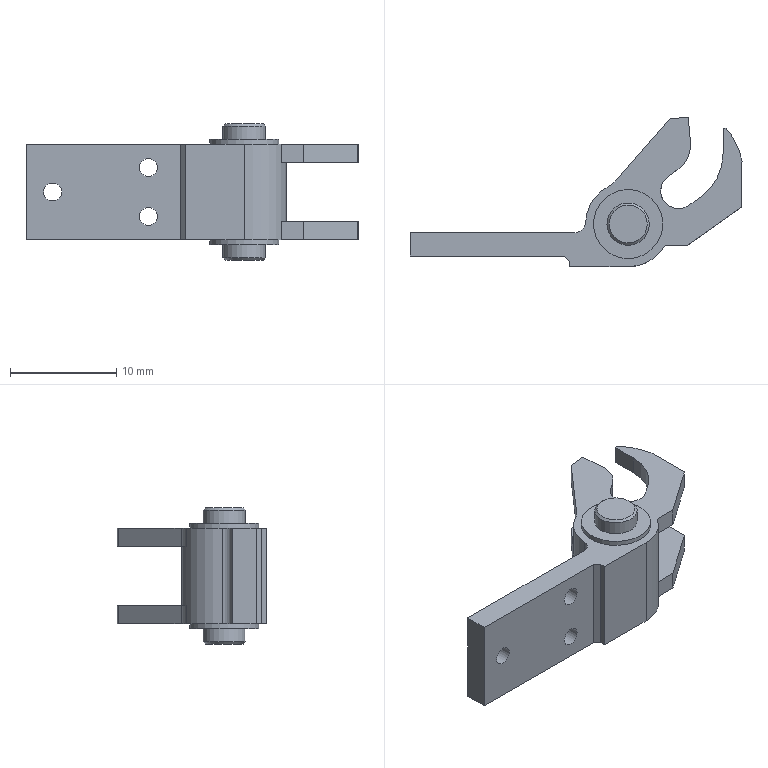NC program | NX | posted with a generic post | part box 31.196 x 14.046 x 12.8 mm
Whole program:
N10 G17 G21 G94 G90
(CAVITY_MILL_COPY_1 , TOOL : D10-ROUGH-LOWSPEED)
N12 T00 M6
N14 G54
N16 G17 G0 G90 X-31.333 Y13.108 B0. C0. S4500 M3
N18 G43 Z18.4 H0
N20 Z8.525
N22 G94 G1 Z6.525 F800.
N24 G3 X-26.548 Y9.559 R5.
N26 G1 X16.744
N28 Y3.023
N30 X6.172
N32 G2 X5.907 Y-3.513 R6.873
N34 G1 X16.744
N36 G3 X21.744 Y1.487 R5.
N38 G1 Z8.525
N40 G0 Z18.4
N42 X-31.548 Y8.022
N44 Z8.525
N46 G1 Z6.525
N48 G3 X-26.548 Y3.023 R5.
N50 G1 X-6.172
N52 G3 X-5.907 Y-3.513 R6.873
N54 G1 X-26.548
N56 G2 X-31.548 Y1.487 R5.
N58 G1 Z8.525
N60 G0 Z18.4
N62 X-31.333 Y13.108
N64 Z6.65
N66 G1 Z4.65
N68 G3 X-26.548 Y9.559 R5.
N70 G1 X16.744
N72 Y3.023
N74 X7.837
N76 G2 X7.63 Y-3.513 R8.4
N78 G1 X16.744
N80 G3 X21.744 Y1.487 R5.
N82 G1 Z6.65
N84 G0 Z18.4
N86 X-31.548 Y8.022
N88 Z6.65
N90 G1 Z4.65
N92 G3 X-26.548 Y3.023 R5.
N94 G1 X-7.837
N96 G3 X-7.63 Y-3.513 R8.4
N98 G1 X-26.548
N100 G2 X-31.548 Y1.487 R5.
N102 G1 Z6.65
N104 G0 Z18.4
N106 M5
(FLOOR_WALL_COPY , TOOL : C5.0)
N108 M6
N110 G54
N112 G17 G0 G90 X-20.306 Y-7.5 B0. C0. S5000 M3
N114 G43 Z18.4 H0
N116 Z6.5
N118 G94 G1 Z4.5 F1000.
N120 G3 X-20.008 Y-5.5 R2.5
N122 G2 X-20.68 Y1.7 R20.75
N124 G1 X-16.915
N126 G3 X-16.086 Y-5.5 R17.
N128 G1 X-12.055
N130 G2 X-13.14 Y1.7 R13.25
N132 G1 X-9.347
N134 G3 X-6.928 Y-6.5 R9.5
N136 G2 X-6.268 Y-8.5 R2.5
N138 G1 Z6.5
N140 G0 Z18.4
N142 X2.915 Y14.324
N144 Z6.5
N146 G1 Z4.5
N148 G3 X4.516 Y12.457 R2.5
N150 G2 X13.196 Y1.195 R13.25
N152 G1 Y0.31
N154 X9.154 Y-2.539
N156 G3 X0.274 Y9.496 R9.5
N158 G1 X0.166 Y5.748
N160 G2 X5.748 Y-0.166 R5.75
N162 X0.166 Y5.748 R-5.75
N164 G3 X2.737 Y8.175 R2.5
N166 G1 X-0.818 Y11.286
N168 Z6.5
N170 G0 Z18.4
N172 M5
(PLANAR_PROFILE_COPY , TOOL : D3-ROUGH-LOWSPEED)
N174 M6
N176 G54
N178 G17 G0 G90 X9.207 Y13.552 B0. C0. S6000 M3
N180 G43 Z16.4 H0
N182 Z6.15
N184 G94 G1 Z4.15 F800.
N186 G41 X7.601 Y11.636
N188 G3 X7.14 Y10.177 R2.
N190 G1 X7.348 Y7.796
N192 G2 X5.542 Y3.907 R4.3
N194 G1 X4.627 Y3.262
N196 G3 X4.584 Y3.018 R0.175
N198 X4.828 Y2.975 R0.175
N200 G1 X5.937 Y3.757
N202 G3 X7.42 Y6.617 R3.5
N204 G1 Y9.
N206 G40
N208 Y9.5
N210 Z6.15
N212 G0 Z16.4
N214 X9.207 Y13.552
N216 Z5.8
N218 G1 Z3.8
N220 G41 X7.601 Y11.636
N222 G3 X7.14 Y10.177 R2.
N224 G1 X7.348 Y7.796
N226 G2 X5.542 Y3.907 R4.3
N228 G1 X4.627 Y3.262
N230 G3 X4.584 Y3.018 R0.175
N232 X4.828 Y2.975 R0.175
N234 G1 X5.937 Y3.757
N236 G3 X7.42 Y6.617 R3.5
N238 G1 Y9.
N240 G40
N242 Y9.5
N244 Z5.8
N246 G0 Z16.4
N248 X9.207 Y13.552
N250 Z5.45
N252 G1 Z3.45
N254 G41 X7.601 Y11.636
N256 G3 X7.14 Y10.177 R2.
N258 G1 X7.348 Y7.796
N260 G2 X5.542 Y3.907 R4.3
N262 G1 X4.627 Y3.262
N264 G3 X4.584 Y3.018 R0.175
N266 X4.828 Y2.975 R0.175
N268 G1 X5.937 Y3.757
N270 G3 X7.42 Y6.617 R3.5
N272 G1 Y9.
N274 G40
N276 Y9.5
N278 Z5.45
N280 G0 Z16.4
N282 X9.207 Y13.552
N284 Z5.1
N286 G1 Z3.1
N288 G41 X7.601 Y11.636
N290 G3 X7.14 Y10.177 R2.
N292 G1 X7.348 Y7.796
N294 G2 X5.542 Y3.907 R4.3
N296 G1 X4.627 Y3.262
N298 G3 X4.584 Y3.018 R0.175
N300 X4.828 Y2.975 R0.175
N302 G1 X5.937 Y3.757
N304 G3 X7.42 Y6.617 R3.5
N306 G1 Y9.
N308 G40
N310 Y9.5
N312 Z5.1
N314 G0 Z16.4
N316 X9.207 Y13.552
N318 Z4.8
N320 G1 Z2.8
N322 G41 X7.601 Y11.636
N324 G3 X7.14 Y10.177 R2.
N326 G1 X7.348 Y7.796
N328 G2 X5.542 Y3.907 R4.3
N330 G1 X4.627 Y3.262
N332 G3 X4.584 Y3.018 R0.175
N334 X4.828 Y2.975 R0.175
N336 G1 X5.937 Y3.757
N338 G3 X7.42 Y6.617 R3.5
N340 G1 Y9.
N342 G40
N344 Y9.5
N346 Z4.8
N348 G0 Z16.4
N350 M5
N352 M2